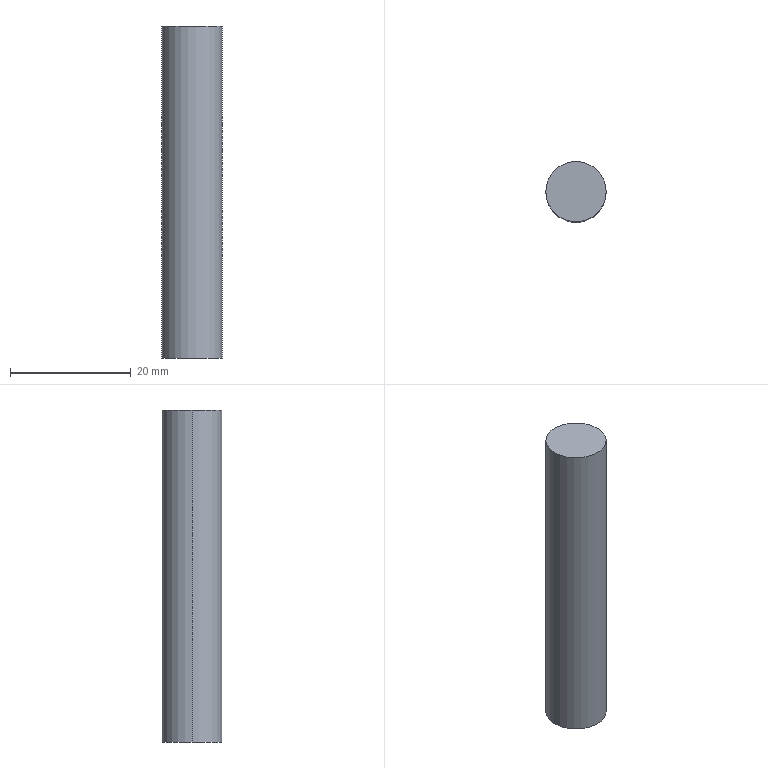Part | SolidWorks | features Extrusion 1 | 1 solid | 4 faces | box 10 x 10 x 55 mm | volume 4320 mm3 | cylinder 2 | plane 2 | commonest cylinder face diameters 10 x2
STEP:
#1=CARTESIAN_POINT('',(5.,0.,55.));
#2=VERTEX_POINT('',#1);
#3=CARTESIAN_POINT('',(-5.,0.,55.));
#4=VERTEX_POINT('',#3);
#5=CARTESIAN_POINT('',(0.,0.,55.));
#6=DIRECTION('',(0.,0.,1.));
#7=DIRECTION('',(1.,0.,0.));
#8=AXIS2_PLACEMENT_3D('',#5,#6,#7);
#9=CIRCLE('',#8,5.);
#10=EDGE_CURVE('',#2,#4,#9,.T.);
#11=ORIENTED_EDGE('',*,*,#10,.F.);
#12=CARTESIAN_POINT('',(5.,0.,0.));
#13=VERTEX_POINT('',#12);
#14=CARTESIAN_POINT('',(5.,0.,55.));
#15=DIRECTION('',(0.,0.,-1.));
#16=VECTOR('',#15,1000.);
#17=LINE('',#14,#16);
#18=EDGE_CURVE('',#2,#13,#17,.T.);
#19=ORIENTED_EDGE('',*,*,#18,.T.);
#20=CARTESIAN_POINT('',(-5.,0.,0.));
#21=VERTEX_POINT('',#20);
#22=CARTESIAN_POINT('',(0.,0.,0.));
#23=DIRECTION('',(0.,0.,1.));
#24=DIRECTION('',(1.,0.,0.));
#25=AXIS2_PLACEMENT_3D('',#22,#23,#24);
#26=CIRCLE('',#25,5.);
#27=EDGE_CURVE('',#13,#21,#26,.T.);
#28=ORIENTED_EDGE('',*,*,#27,.T.);
#29=CARTESIAN_POINT('',(-5.,0.,55.));
#30=DIRECTION('',(0.,0.,-1.));
#31=VECTOR('',#30,1000.);
#32=LINE('',#29,#31);
#33=EDGE_CURVE('',#4,#21,#32,.T.);
#34=ORIENTED_EDGE('',*,*,#33,.F.);
#35=EDGE_LOOP('',(#11,#19,#28,#34));
#36=FACE_OUTER_BOUND('',#35,.T.);
#37=CARTESIAN_POINT('',(0.,0.,55.));
#38=DIRECTION('',(0.,0.,-1.));
#39=DIRECTION('',(-1.,0.,0.));
#40=AXIS2_PLACEMENT_3D('',#37,#38,#39);
#41=CYLINDRICAL_SURFACE('',#40,5.);
#42=ADVANCED_FACE('',(#36),#41,.T.);
#43=ORIENTED_EDGE('',*,*,#18,.F.);
#44=CARTESIAN_POINT('',(0.,0.,55.));
#45=DIRECTION('',(0.,0.,1.));
#46=DIRECTION('',(1.,0.,0.));
#47=AXIS2_PLACEMENT_3D('',#44,#45,#46);
#48=CIRCLE('',#47,5.);
#49=EDGE_CURVE('',#4,#2,#48,.T.);
#50=ORIENTED_EDGE('',*,*,#49,.F.);
#51=ORIENTED_EDGE('',*,*,#33,.T.);
#52=CARTESIAN_POINT('',(0.,0.,0.));
#53=DIRECTION('',(0.,0.,1.));
#54=DIRECTION('',(1.,0.,0.));
#55=AXIS2_PLACEMENT_3D('',#52,#53,#54);
#56=CIRCLE('',#55,5.);
#57=EDGE_CURVE('',#21,#13,#56,.T.);
#58=ORIENTED_EDGE('',*,*,#57,.T.);
#59=EDGE_LOOP('',(#43,#50,#51,#58));
#60=FACE_OUTER_BOUND('',#59,.T.);
#61=CARTESIAN_POINT('',(0.,0.,55.));
#62=DIRECTION('',(0.,0.,-1.));
#63=DIRECTION('',(-1.,0.,0.));
#64=AXIS2_PLACEMENT_3D('',#61,#62,#63);
#65=CYLINDRICAL_SURFACE('',#64,5.);
#66=ADVANCED_FACE('',(#60),#65,.T.);
#67=ORIENTED_EDGE('',*,*,#49,.T.);
#68=ORIENTED_EDGE('',*,*,#10,.T.);
#69=EDGE_LOOP('',(#67,#68));
#70=FACE_OUTER_BOUND('',#69,.T.);
#71=CARTESIAN_POINT('',(0.,0.,55.));
#72=DIRECTION('',(0.,0.,1.));
#73=DIRECTION('',(1.,0.,0.));
#74=AXIS2_PLACEMENT_3D('',#71,#72,#73);
#75=PLANE('',#74);
#76=ADVANCED_FACE('',(#70),#75,.T.);
#77=ORIENTED_EDGE('',*,*,#57,.F.);
#78=ORIENTED_EDGE('',*,*,#27,.F.);
#79=EDGE_LOOP('',(#77,#78));
#80=FACE_OUTER_BOUND('',#79,.T.);
#81=CARTESIAN_POINT('',(0.,0.,0.));
#82=DIRECTION('',(0.,0.,1.));
#83=DIRECTION('',(1.,0.,0.));
#84=AXIS2_PLACEMENT_3D('',#81,#82,#83);
#85=PLANE('',#84);
#86=ADVANCED_FACE('',(#80),#85,.F.);
#87=CLOSED_SHELL('',(#42,#66,#76,#86));
#88=MANIFOLD_SOLID_BREP('',#87);
#89=CARTESIAN_POINT('',(0.,0.,0.));
#90=DIRECTION('',(0.,0.,1.));
#91=DIRECTION('',(1.,0.,0.));
#92=AXIS2_PLACEMENT_3D('',#89,#90,#91);
#93=(LENGTH_UNIT()NAMED_UNIT(*)SI_UNIT(.MILLI.,.METRE.));
#94=UNCERTAINTY_MEASURE_WITH_UNIT(LENGTH_MEASURE(0.00001),#93,'','');
#95=(NAMED_UNIT(*)PLANE_ANGLE_UNIT()SI_UNIT($,.RADIAN.));
#96=(NAMED_UNIT(*)SI_UNIT($,.STERADIAN.)SOLID_ANGLE_UNIT());
#97=(GEOMETRIC_REPRESENTATION_CONTEXT(3)GLOBAL_UNCERTAINTY_ASSIGNED_CONTEXT((#94))GLOBAL_UNIT_ASSIGNED_CONTEXT((#93,#95,#96))REPRESENTATION_CONTEXT('',''));
#98=ADVANCED_BREP_SHAPE_REPRESENTATION('',(#88,#92),#97);